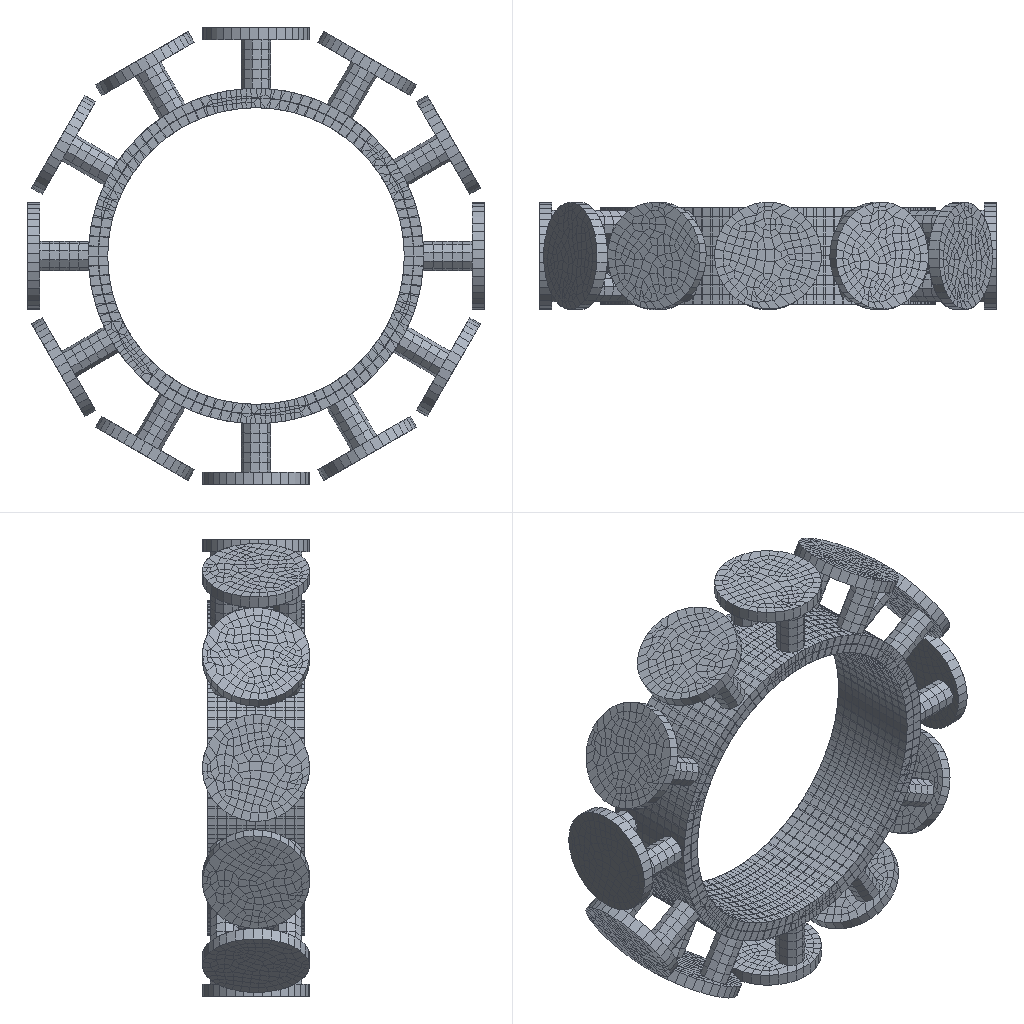Simulation study | abaqus
Set-up summary:
category,name,step,type,value,unit,region
solver,abaqus
solver,version,,,Abaqus/Explicit 2020
units,not stated in the deck,,not stated
analysis,deck,,transient,transient
load_step,Step-1,Step-1,transient
load_step,requested,,,1
mesh,nodes,,,21948
mesh,elements,,,16928
element_type,S4R,,shell,11811
element_type,C3D8R,,solid,5117
load,load commands in deck,,count,12
bc,support commands in deck,,count,5
material,CON,,in results
material,FRP,,in results
material,MATERIAL-3,,in results
check,setup vs results,,match,"per instance, exact: element labels, types and connectivity; labels of the nodes the elements use; coordinates of those nodes at SINGLE_PRECISION in 19 of 19 instance(s)"
Abaqus input file, long lists of numbers shortened:
*Heading
** Job name: Job-1 Model name: Model-1
** Generated by: Abaqus/CAE 2020
*Preprint, echo=NO, model=NO, history=NO, contact=NO
**
** PARTS
**
*Part, name=con
*Node
      1,         610.,   1219.589,           0.
      2,         650.,   1219.589,           0.
** (916 more lines like these left out)
*Element, type=C3D8R
  1,  10,  11,  14,  13,   1,   2,   5,   4
  2,  11,  12,  15,  14,   2,   3,   6,   5
** (406 more lines like these left out)
*Nset, nset=Set-1, generate
   1,  918,    1
*Elset, elset=Set-1, generate
   1,  408,    1
** Section: con
*Solid Section, elset=Set-1, material=con
,
*End Part
**
*Part, name=frp
*Node
      1,   666.024,    1000.002,           0.
      2,   666.024,    1160.002,           0.
** (8318 more lines like these left out)
*Element, type=S4R
   1,   48,   41,    6,    1
   2,   41,   42,    7,    6
** (8318 more lines like these left out)
*Nset, nset=Set-3, generate
    1,  8320,     1
*Elset, elset=Set-3, generate
    1,  8320,     1
** Section: Section-1
*Shell Section, elset=Set-3, material=frp
7., 5
*End Part
**
*Part, name=gangban
*Node
      1,         610.,   1059.589,           0.
      2,         610.,   979.589,           0.
** (3081 more lines like these left out)
*Element, type=S4R
  1,    1,   13, 1241,  108
  2,   13,   14, 1242, 1241
** (3489 more lines like these left out)
*Nset, nset=Set-3, generate
    1,  3083,     1
*Elset, elset=Set-3, generate
    1,  3491,     1
** Section: Section-1
*Shell Section, elset=Set-3, material=frp
7., 5
*End Part
**
*Part, name=m1
*Node
      1,         890.,   1007.07,  -46.852
      2,   688.407,   1007.07,  -46.852
** (478 more lines like these left out)
*Element, type=C3D8R
 1, 434, 437, 435, 433, 114, 117, 115, 113
 2, 438, 434, 433, 436, 118, 114, 113, 116
** (239 more lines like these left out)
*Nset, nset=Set-1, generate
   1,  480,    1
*Elset, elset=Set-1, generate
   1,  241,    1
** Section: m
*Solid Section, elset=Set-1, material=Material-3
,
*End Part
**
*Part, name=m2
*Node
      1,   747.337,   1007.07,  -485.575
      2,   572.752,   1007.07,   -384.779
** (516 more lines like these left out)
*Element, type=C3D8R
 1, 119,  12,  11, 120, 453, 130, 129, 454
 2, 114,  10,   9, 121, 448, 128, 127, 455
** (273 more lines like these left out)
*Nset, nset=Set-3, generate
   1,  518,    1
*Elset, elset=Set-3, generate
   1,  275,    1
** Section: m
*Solid Section, elset=Set-3, material=Material-3
,
*End Part
**
*Part, name=m3
*Node
      1,   404.425,   1007.07,   -794.189
      2,   303.629,   1007.07,  -619.604
** (537 more lines like these left out)
*Element, type=C3D8R
 1, 119,  12,  11, 120, 462, 130, 129, 463
 2, 114,  10,   9, 121, 457, 128, 127, 464
** (291 more lines like these left out)
*Nset, nset=Set-1, generate
   1,  539,    1
*Elset, elset=Set-1, generate
   1,  293,    1
** Section: m
*Solid Section, elset=Set-1, material=Material-3
,
*End Part
**
*Part, name=m4
*Node
      1,  -46.852,   1007.07,        -890.
      2,  -46.852,   1007.07,  -688.407
** (478 more lines like these left out)
*Element, type=C3D8R
 1, 434, 437, 435, 433, 114, 117, 115, 113
 2, 438, 434, 433, 436, 118, 114, 113, 116
** (239 more lines like these left out)
*Nset, nset=Set-1, generate
   1,  480,    1
*Elset, elset=Set-1, generate
   1,  241,    1
** Section: m
*Solid Section, elset=Set-1, material=Material-3
,
*End Part
**
*Part, name=m5
*Node
      1,  -485.575,   1007.07,  -747.337
      2,   -384.779,   1007.07,  -572.752
** (487 more lines like these left out)
*Element, type=C3D8R
 1, 430, 123, 124, 434, 113,   8,   9, 117
 2, 432, 437, 433, 431, 115, 120, 116, 114
** (251 more lines like these left out)
*Nset, nset=Set-1, generate
   1,  489,    1
*Elset, elset=Set-1, generate
   1,  253,    1
** Section: m
*Solid Section, elset=Set-1, material=Material-3
,
*End Part
**
*Part, name=m6
*Node
      1,   -794.189,   1007.07,  -404.425
      2,  -619.604,   1007.07,  -303.629
** (466 more lines like these left out)
*Element, type=C3D8R
 1, 429, 118, 119, 120, 113,   8,   9,  10
 2, 125, 431, 430, 124,  15, 115, 114,  14
** (228 more lines like these left out)
*Nset, nset=Set-1, generate
   1,  468,    1
*Elset, elset=Set-1, generate
   1,  230,    1
** Section: m
*Solid Section, elset=Set-1, material=Material-3
,
*End Part
**
*Part, name=m7
*Node
      1,        -890.,   1007.07,   46.852
      2,  -688.407,   1007.07,   46.852
** (462 more lines like these left out)
*Element, type=C3D8R
 1, 118, 119, 427, 425,   8,   9, 115, 113
 2, 428, 426, 425, 427, 116, 114, 113, 115
** (226 more lines like these left out)
*Nset, nset=Set-1, generate
   1,  464,    1
*Elset, elset=Set-1, generate
   1,  228,    1
** Section: m
*Solid Section, elset=Set-1, material=Material-3
,
*End Part
**
*Part, name=m8
*Node
      1,  -747.337,   1007.07,   485.575
      2,  -572.752,   1007.07,    384.779
** (516 more lines like these left out)
*Element, type=C3D8R
 1, 119,  12,  11, 120, 453, 130, 129, 454
 2,  10,   9, 121, 114, 128, 127, 455, 448
** (273 more lines like these left out)
*Nset, nset=Set-1, generate
   1,  518,    1
*Elset, elset=Set-1, generate
   1,  275,    1
** Section: m
*Solid Section, elset=Set-1, material=Material-3
,
*End Part
**
*Part, name=m9
*Node
      1,  -404.425,   1007.07,    794.189
      2,  -303.629,   1007.07,   619.604
** (468 more lines like these left out)
*Element, type=C3D8R
 1, 423, 120, 121, 426, 113,   8,   9, 116
 2, 428, 426, 123, 124, 118, 116,  11,  12
** (234 more lines like these left out)
*Nset, nset=Set-1, generate
   1,  470,    1
*Elset, elset=Set-1, generate
   1,  236,    1
** Section: m
*Solid Section, elset=Set-1, material=Material-3
,
*End Part
**
*Part, name=m10
*Node
      1,   46.852,   1007.07,         890.
      2,   46.852,   1007.07,   688.407
** (541 more lines like these left out)
*Element, type=C3D8R
 1, 113, 123, 119, 120, 460, 470, 466, 467
 2, 114,  10,   9, 121, 461, 128, 127, 468
** (293 more lines like these left out)
*Nset, nset=Set-1, generate
   1,  543,    1
*Elset, elset=Set-1, generate
   1,  295,    1
** Section: m
*Solid Section, elset=Set-1, material=Material-3
,
*End Part
**
*Part, name=m11
*Node
      1,   485.575,   1007.07,   747.337
      2,    384.779,   1007.07,   572.752
** (516 more lines like these left out)
*Element, type=C3D8R
 1, 119,  12,  11, 120, 453, 130, 129, 454
 2, 114,  10,   9, 121, 448, 128, 127, 455
** (273 more lines like these left out)
*Nset, nset=Set-1, generate
   1,  518,    1
*Elset, elset=Set-1, generate
   1,  275,    1
** Section: m
*Solid Section, elset=Set-1, material=Material-3
,
*End Part
**
*Part, name=m12
*Node
      1,    794.189,   1007.07,   404.425
      2,   619.604,   1007.07,   303.629
** (466 more lines like these left out)
*Element, type=C3D8R
 1, 421, 120, 121, 424, 113,   8,   9, 116
 2, 426, 424, 123, 124, 118, 116,  11,  12
** (233 more lines like these left out)
*Nset, nset=Set-1, generate
   1,  468,    1
*Elset, elset=Set-1, generate
   1,  235,    1
** Section: m
*Solid Section, elset=Set-1, material=Material-3
,
*End Part
**
**
** ASSEMBLY
**
*Assembly, name=Assembly
**
*Instance, name=con-1, part=con
*End Instance
**
*Instance, name=frp-1, part=frp
*End Instance
**
*Instance, name=gangban-1, part=gangban
*End Instance
**
*Instance, name=con-1-lin-1-2, part=con
          0.,         -80.,           0.
*End Instance
**
*Instance, name=con-1-lin-1-3, part=con
          0.,        -160.,           0.
*End Instance
**
*Instance, name=con-1-lin-1-4, part=con
          0.,        -240.,           0.
*End Instance
**
*Instance, name=con-1-lin-1-5, part=con
          0.,        -320.,           0.
*End Instance
**
*Instance, name=m1-1, part=m1
*End Instance
**
*Instance, name=m2-1, part=m2
*End Instance
**
*Instance, name=m3-1, part=m3
*End Instance
**
*Instance, name=m4-1, part=m4
*End Instance
**
*Instance, name=m5-1, part=m5
*End Instance
**
*Instance, name=m6-1, part=m6
*End Instance
**
*Instance, name=m7-1, part=m7
*End Instance
**
*Instance, name=m8-1, part=m8
*End Instance
**
*Instance, name=m9-1, part=m9
*End Instance
**
*Instance, name=m10-1, part=m10
*End Instance
**
*Instance, name=m11-1, part=m11
*End Instance
**
*Instance, name=m12-1, part=m12
*End Instance
**
*Node
      1,         470.,   1099.589,   814.064
*Node
      2,   814.064,   1099.589,         470.
*Node
      3,         940.,   1099.589, 1.34711146e-14
*Node
      4,   814.064,   1099.589,        -470.
*Node
      5,         470.,   1099.589,  -814.064
*Node
      6, 7.10295131e-14,   1099.589,        -940.
*Node
      7,        -470.,   1099.589,  -814.064
*Node
      8,  -814.064,   1099.589,        -470.
*Node
      9,        -940.,   1099.589, -1.28587909e-13
*Node
     10,  -814.064,   1099.589,         470.
*Node
     11,        -470.,   1099.589,   814.064
*Node
     12, -1.86146319e-13,   1099.589,         940.
*Node
     13,           0.,   1059.589, -3.73517271e-14
*Nset, nset=Set-3, instance=con-1
   7,   8,   9,  16,  17,  18,  25,  26,  27,  34,  35,  36,  43,  44,  45,  52
  53,  54,  61,  62,  63,  70,  71,  72,  79,  80,  81,  88,  89,  90,  97,  98
** (18 more lines like these left out)
*Elset, elset=Set-3, instance=con-1
   3,   4,   7,   8,  11,  12,  15,  16,  19,  20,  23,  24,  27,  28,  31,  32
  35,  36,  39,  40,  43,  44,  47,  48,  51,  52,  55,  56,  59,  60,  63,  64
** (11 more lines like these left out)
*Nset, nset=Set-4, instance=m1-1
   4,   5,  34,  35,  36,  37,  38,  39,  40,  41,  42,  43,  44,  45,  46,  47
  48,  49,  50,  51,  52,  53,  54,  55,  56,  57,  58,  59,  60,  61,  62,  63
** (3 more lines like these left out)
*Nset, nset=Set-4, instance=m2-1
   4,   5,  34,  35,  36,  37,  38,  39,  40,  41,  42,  43,  44,  45,  46,  47
  48,  49,  50,  51,  52,  53,  54,  55,  56,  57,  58,  59,  60,  61,  62,  63
** (3 more lines like these left out)
*Nset, nset=Set-4, instance=m4-1
   4,   5,  34,  35,  36,  37,  38,  39,  40,  41,  42,  43,  44,  45,  46,  47
  48,  49,  50,  51,  52,  53,  54,  55,  56,  57,  58,  59,  60,  61,  62,  63
** (3 more lines like these left out)
*Nset, nset=Set-4, instance=m6-1
   4,   5,  34,  35,  36,  37,  38,  39,  40,  41,  42,  43,  44,  45,  46,  47
  48,  49,  50,  51,  52,  53,  54,  55,  56,  57,  58,  59,  60,  61,  62,  63
** (3 more lines like these left out)
*Nset, nset=Set-4, instance=m10-1
   4,   5,  34,  35,  36,  37,  38,  39,  40,  41,  42,  43,  44,  45,  46,  47
  48,  49,  50,  51,  52,  53,  54,  55,  56,  57,  58,  59,  60,  61,  62,  63
** (3 more lines like these left out)
*Nset, nset=Set-4, instance=m8-1
   4,   5,  34,  35,  36,  37,  38,  39,  40,  41,  42,  43,  44,  45,  46,  47
  48,  49,  50,  51,  52,  53,  54,  55,  56,  57,  58,  59,  60,  61,  62,  63
** (3 more lines like these left out)
*Nset, nset=Set-4, instance=m12-1
   4,   5,  34,  35,  36,  37,  38,  39,  40,  41,  42,  43,  44,  45,  46,  47
  48,  49,  50,  51,  52,  53,  54,  55,  56,  57,  58,  59,  60,  61,  62,  63
** (3 more lines like these left out)
*Nset, nset=Set-4, instance=m3-1
   4,   5,  34,  35,  36,  37,  38,  39,  40,  41,  42,  43,  44,  45,  46,  47
  48,  49,  50,  51,  52,  53,  54,  55,  56,  57,  58,  59,  60,  61,  62,  63
** (3 more lines like these left out)
*Nset, nset=Set-4, instance=m7-1
   4,   5,  34,  35,  36,  37,  38,  39,  40,  41,  42,  43,  44,  45,  46,  47
  48,  49,  50,  51,  52,  53,  54,  55,  56,  57,  58,  59,  60,  61,  62,  63
** (3 more lines like these left out)
*Nset, nset=Set-4, instance=m11-1
   4,   5,  34,  35,  36,  37,  38,  39,  40,  41,  42,  43,  44,  45,  46,  47
  48,  49,  50,  51,  52,  53,  54,  55,  56,  57,  58,  59,  60,  61,  62,  63
** (3 more lines like these left out)
*Nset, nset=Set-4, instance=m5-1
   4,   5,  34,  35,  36,  37,  38,  39,  40,  41,  42,  43,  44,  45,  46,  47
  48,  49,  50,  51,  52,  53,  54,  55,  56,  57,  58,  59,  60,  61,  62,  63
** (3 more lines like these left out)
*Nset, nset=Set-4, instance=m9-1
   4,   5,  34,  35,  36,  37,  38,  39,  40,  41,  42,  43,  44,  45,  46,  47
  48,  49,  50,  51,  52,  53,  54,  55,  56,  57,  58,  59,  60,  61,  62,  63
** (3 more lines like these left out)
*Elset, elset=Set-4, instance=m1-1
  77,  80,  82,  83,  84,  86,  88,  90,  91,  92,  98,  99, 100, 104, 105, 106
 107, 109, 111, 112, 113, 116, 118, 122, 129, 130, 131, 132, 133, 134, 136, 137
** (1 more lines like these left out)
*Elset, elset=Set-4, instance=m2-1
 101, 106, 107, 108, 109, 110, 111, 112, 113, 115, 117, 122, 123, 130, 131, 132
 133, 134, 138, 141, 143, 147, 153, 154, 156, 157, 158, 159, 160, 161, 164, 165
** (1 more lines like these left out)
*Elset, elset=Set-4, instance=m4-1
  77,  80,  82,  83,  84,  87,  89,  91,  92,  93,  99, 100, 101, 104, 105, 106
 107, 109, 111, 112, 113, 116, 117, 121, 129, 130, 131, 132, 133, 134, 136, 137
** (1 more lines like these left out)
*Elset, elset=Set-4, instance=m6-1
  52,  53,  61,  62,  66,  67,  68,  70,  71,  72,  73,  74,  76,  80,  84,  88
  89,  92,  93,  94,  97, 101, 107, 112, 113, 114, 117, 118, 119, 121, 122, 124
** (1 more lines like these left out)
*Elset, elset=Set-4, instance=m10-1
 103, 111, 112, 114, 115, 116, 118, 120, 123, 124, 126, 131, 133, 137, 138, 139
 140, 142, 145, 148, 150, 153, 160, 161, 162, 163, 164, 165, 166, 167, 168, 170
** (1 more lines like these left out)
*Elset, elset=Set-4, instance=m8-1
 100, 105, 106, 107, 108, 109, 110, 111, 112, 113, 115, 120, 121, 122, 130, 131
 133, 134, 138, 142, 145, 153, 154, 155, 156, 157, 158, 159, 161, 162, 165, 166
** (1 more lines like these left out)
*Elset, elset=Set-4, instance=m12-1
  62,  63,  71,  75,  76,  77,  79,  80,  81,  82,  83,  85,  89,  91,  94,  97
  98, 101, 102, 103, 106, 110, 115, 122, 123, 124, 125, 126, 129, 130, 134, 135
** (1 more lines like these left out)
*Elset, elset=Set-4, instance=m3-1
  95,  96, 104, 109, 110, 111, 113, 114, 115, 116, 118, 123, 124, 127, 131, 132
 135, 136, 138, 141, 145, 149, 153, 158, 159, 161, 162, 163, 165, 166, 168, 169
** (1 more lines like these left out)
*Elset, elset=Set-4, instance=m7-1
  67,  70,  72,  73,  74,  77,  79,  81,  82,  83,  89,  90,  91,  94,  95,  96
  97,  99, 100, 101, 102, 105, 106, 111, 118, 119, 120, 122, 123, 124, 126, 127
** (1 more lines like these left out)
*Elset, elset=Set-4, instance=m11-1
 101, 106, 107, 109, 110, 111, 112, 113, 115, 117, 122, 123, 124, 131, 132, 133
 134, 138, 141, 145, 147, 152, 153, 154, 155, 157, 159, 160, 161, 162, 165, 166
** (1 more lines like these left out)
*Elset, elset=Set-4, instance=m5-1
  86,  91,  92,  93,  94,  96,  97,  98, 100, 102, 106, 115, 116, 117, 118, 119
 121, 124, 126, 133, 137, 138, 140, 141, 142, 143, 144, 145, 146, 147, 151, 152
** (1 more lines like these left out)
*Elset, elset=Set-4, instance=m9-1
  62,  63,  71,  75,  76,  77,  78,  80,  81,  82,  83,  85,  87,  91,  93,  99
 100, 103, 104, 105, 108, 112, 117, 120, 124, 125, 126, 127, 130, 131, 135, 136
** (1 more lines like these left out)
*Nset, nset=Set-30
 13,
*Nset, nset=b_Set-5, instance=m11-1, generate
   1,  518,    1
*Elset, elset=b_Set-5, instance=m11-1, generate
   1,  275,    1
*Nset, nset=b_Set-7, instance=m12-1, generate
   1,  468,    1
*Elset, elset=b_Set-7, instance=m12-1, generate
   1,  235,    1
*Nset, nset=b_Set-9, instance=m1-1, generate
   1,  480,    1
*Elset, elset=b_Set-9, instance=m1-1, generate
   1,  241,    1
*Nset, nset=b_Set-11, instance=m2-1, generate
   1,  518,    1
*Elset, elset=b_Set-11, instance=m2-1, generate
   1,  275,    1
*Nset, nset=b_Set-13, instance=m3-1, generate
   1,  539,    1
*Elset, elset=b_Set-13, instance=m3-1, generate
   1,  293,    1
*Nset, nset=b_Set-15, instance=m4-1, generate
   1,  480,    1
*Elset, elset=b_Set-15, instance=m4-1, generate
   1,  241,    1
*Nset, nset=b_Set-17, instance=m5-1, generate
   1,  489,    1
*Elset, elset=b_Set-17, instance=m5-1, generate
   1,  253,    1
*Nset, nset=b_Set-19, instance=m6-1, generate
   1,  468,    1
*Elset, elset=b_Set-19, instance=m6-1, generate
   1,  230,    1
*Nset, nset=b_Set-21, instance=m7-1, generate
   1,  464,    1
*Elset, elset=b_Set-21, instance=m7-1, generate
   1,  228,    1
*Nset, nset=b_Set-23, instance=m8-1, generate
   1,  518,    1
*Elset, elset=b_Set-23, instance=m8-1, generate
   1,  275,    1
*Nset, nset=b_Set-25, instance=m9-1, generate
   1,  470,    1
*Elset, elset=b_Set-25, instance=m9-1, generate
   1,  236,    1
*Nset, nset=b_Set-27, instance=m10-1, generate
   1,  543,    1
*Elset, elset=b_Set-27, instance=m10-1, generate
   1,  295,    1
*Nset, nset=m_Set-1, instance=frp-1, generate
    1,  8320,     1
*Elset, elset=m_Set-1, instance=frp-1, generate
    1,  8320,     1
*Nset, nset=m_Set-29
 13,
*Nset, nset=s_Set-1, instance=con-1, generate
   1,  918,    1
*Nset, nset=s_Set-1, instance=con-1-lin-1-2, generate
   1,  918,    1
*Nset, nset=s_Set-1, instance=con-1-lin-1-3, generate
   1,  918,    1
*Nset, nset=s_Set-1, instance=con-1-lin-1-5, generate
   1,  918,    1
*Nset, nset=s_Set-1, instance=con-1-lin-1-4, generate
   1,  918,    1
*Elset, elset=s_Set-1, instance=con-1, generate
   1,  408,    1
*Elset, elset=s_Set-1, instance=con-1-lin-1-2, generate
   1,  408,    1
*Elset, elset=s_Set-1, instance=con-1-lin-1-3, generate
   1,  408,    1
*Elset, elset=s_Set-1, instance=con-1-lin-1-5, generate
   1,  408,    1
*Elset, elset=s_Set-1, instance=con-1-lin-1-4, generate
   1,  408,    1
*Nset, nset=_PickedSet98, internal
 1,
*Nset, nset=_PickedSet100, internal
 2,
*Nset, nset=_PickedSet102, internal
 3,
*Nset, nset=_PickedSet104, internal
 4,
*Nset, nset=_PickedSet106, internal
 5,
*Nset, nset=_PickedSet108, internal
 6,
*Nset, nset=_PickedSet110, internal
 7,
*Nset, nset=_PickedSet112, internal
 8,
*Nset, nset=_PickedSet114, internal
 9,
*Nset, nset=_PickedSet116, internal
 10,
*Nset, nset=_PickedSet118, internal
 11,
*Nset, nset=_PickedSet120, internal
 12,
*Elset, elset=_Surf-1_S1, internal, instance=m10-1, generate
  81,  214,    1
*Elset, elset=_Surf-1_S2, internal, instance=m10-1, generate
 215,  230,    1
*Surface, type=ELEMENT, name=Surf-1
_Surf-1_S1, S1
_Surf-1_S2, S2
*Elset, elset=_Surf-2_S2, internal, instance=m9-1
  51,  52,  53,  54,  55,  56,  57,  58,  59,  60, 177, 178, 179, 180, 181, 182
 183, 184, 185, 186
*Elset, elset=_Surf-2_S1, internal, instance=m9-1, generate
  61,  176,    1
*Surface, type=ELEMENT, name=Surf-2
_Surf-2_S2, S2
_Surf-2_S1, S1
*Elset, elset=_Surf-3_S1, internal, instance=m8-1, generate
  81,  209,    1
*Elset, elset=_Surf-3_S2, internal, instance=m8-1, generate
 210,  225,    1
*Surface, type=ELEMENT, name=Surf-3
_Surf-3_S1, S1
_Surf-3_S2, S2
*Elset, elset=_Surf-4_S2, internal, instance=m7-1
  41,  42,  43,  44,  45,  46,  47,  48,  49,  50, 171, 172, 173, 174, 175, 176
 177, 178
*Elset, elset=_Surf-4_S1, internal, instance=m7-1, generate
  51,  170,    1
*Surface, type=ELEMENT, name=Surf-4
_Surf-4_S2, S2
_Surf-4_S1, S1
*Elset, elset=_Surf-5_S2, internal, instance=m6-1
  41,  42,  43,  44,  45,  46,  47,  48,  49,  50, 173, 174, 175, 176, 177, 178
 179, 180
*Elset, elset=_Surf-5_S1, internal, instance=m6-1, generate
  51,  172,    1
*Surface, type=ELEMENT, name=Surf-5
_Surf-5_S2, S2
_Surf-5_S1, S1
*Elset, elset=_Surf-6_S2, internal, instance=m5-1
  66,  67,  68,  69,  70,  71,  72,  73,  74,  75, 191, 192, 193, 194, 195, 196
 197, 198, 199, 200, 201, 202, 203
*Elset, elset=_Surf-6_S1, internal, instance=m5-1, generate
  76,  190,    1
*Surface, type=ELEMENT, name=Surf-6
_Surf-6_S2, S2
_Surf-6_S1, S1
*Elset, elset=_Surf-7_S2, internal, instance=m4-1
  51,  52,  53,  54,  55,  56,  57,  58,  59,  60, 182, 183, 184, 185, 186, 187
 188, 189, 190, 191
*Elset, elset=_Surf-7_S1, internal, instance=m4-1, generate
  61,  181,    1
*Surface, type=ELEMENT, name=Surf-7
_Surf-7_S2, S2
_Surf-7_S1, S1
*Elset, elset=_Surf-8_S1, internal, instance=m3-1, generate
  81,  212,    1
*Elset, elset=_Surf-8_S2, internal, instance=m3-1, generate
 213,  228,    1
*Surface, type=ELEMENT, name=Surf-8
_Surf-8_S1, S1
_Surf-8_S2, S2
*Elset, elset=_Surf-9_S1, internal, instance=m2-1, generate
  81,  209,    1
*Elset, elset=_Surf-9_S2, internal, instance=m2-1, generate
 210,  225,    1
*Surface, type=ELEMENT, name=Surf-9
_Surf-9_S1, S1
_Surf-9_S2, S2
*Elset, elset=_Surf-10_S2, internal, instance=m1-1
  51,  52,  53,  54,  55,  56,  57,  58,  59,  60, 182, 183, 184, 185, 186, 187
 188, 189, 190, 191
*Elset, elset=_Surf-10_S1, internal, instance=m1-1, generate
  61,  181,    1
*Surface, type=ELEMENT, name=Surf-10
_Surf-10_S2, S2
_Surf-10_S1, S1
*Elset, elset=_Surf-11_S2, internal, instance=m12-1
  51,  52,  53,  54,  55,  56,  57,  58,  59,  60, 176, 177, 178, 179, 180, 181
 182, 183, 184, 185
*Elset, elset=_Surf-11_S1, internal, instance=m12-1, generate
  61,  175,    1
*Surface, type=ELEMENT, name=Surf-11
_Surf-11_S2, S2
_Surf-11_S1, S1
*Elset, elset=_Surf-12_S1, internal, instance=m11-1, generate
  81,  209,    1
*Elset, elset=_Surf-12_S2, internal, instance=m11-1, generate
 210,  225,    1
*Surface, type=ELEMENT, name=Surf-12
_Surf-12_S1, S1
_Surf-12_S2, S2
*Elset, elset=_s_Surf-14_SPOS, internal, instance=gangban-1, generate
 3017,  3491,     1
*Surface, type=ELEMENT, name=s_Surf-14
_s_Surf-14_SPOS, SPOS
*Elset, elset=_shuchu_SPOS, internal, instance=gangban-1
  193,  194,  195,  196,  197,  198,  199,  200,  201,  202,  203,  204,  205,  206,  207,  208
  209,  210,  211,  212,  213,  214,  215,  216,  217,  218,  219,  220,  221,  222,  223,  224
** (66 more lines like these left out)
*Surface, type=ELEMENT, name=shuchu
_shuchu_SPOS, SPOS
** Constraint: Constraint-1
*Embedded Element, host elset=s_Set-1
m_Set-1
** Constraint: Constraint-2
*Rigid Body, ref node=_PickedSet98, elset=b_Set-5
** Constraint: Constraint-3
*Rigid Body, ref node=_PickedSet100, elset=b_Set-7
** Constraint: Constraint-4
*Rigid Body, ref node=_PickedSet102, elset=b_Set-9
** Constraint: Constraint-5
*Rigid Body, ref node=_PickedSet104, elset=b_Set-11
** Constraint: Constraint-6
*Rigid Body, ref node=_PickedSet106, elset=b_Set-13
** Constraint: Constraint-7
*Rigid Body, ref node=_PickedSet108, elset=b_Set-15
** Constraint: Constraint-8
*Rigid Body, ref node=_PickedSet110, elset=b_Set-17
** Constraint: Constraint-9
*Rigid Body, ref node=_PickedSet112, elset=b_Set-19
** Constraint: Constraint-10
*Rigid Body, ref node=_PickedSet114, elset=b_Set-21
** Constraint: Constraint-11
*Rigid Body, ref node=_PickedSet116, elset=b_Set-23
** Constraint: Constraint-12
*Rigid Body, ref node=_PickedSet118, elset=b_Set-25
** Constraint: Constraint-13
*Rigid Body, ref node=_PickedSet120, elset=b_Set-27
** Constraint: Constraint-SHUCHU
*Coupling, constraint name=Constraint-SHUCHU, ref node=m_Set-29, surface=s_Surf-14
*Kinematic
*End Assembly
*Amplitude, name=Amp-1
             0.,              0.,             0.5,              1.
**
** MATERIALS
**
*Material, name=Material-3
*Density
 7.8e-09,
*Elastic
180000., 0.3
*Plastic
347.,0.
*Material, name=con
*Density
 2.2e-09,
*Elastic
35900., 0.22
*Plastic
60.,0.
*Material, name=frp
*Density
 1.5e-09,
*Elastic, type=ENGINEERING CONSTANTS
11810.,11200.,11810.,  0.24,  0.23,  0.23, 7800., 8900.
 8900.,
**
** INTERACTION PROPERTIES
**
*Surface Interaction, name=IntProp-1
*Friction
 0.2,
*Surface Behavior, pressure-overclosure=HARD
**
** INTERACTIONS
**
** Interaction: Int-1
*Contact, op=NEW
*Contact Inclusions, ALL EXTERIOR
*Contact Property Assignment
 ,  , IntProp-1
** ----------------------------------------------------------------
**
** STEP: Step-1
**
*Step, name=Step-1, nlgeom=YES
*Dynamic, Explicit
, 0.5
*Bulk Viscosity
0.06, 1.2
** Mass Scaling: Semi-Automatic
**               Whole Model
*Fixed Mass Scaling, factor=50.
**
** BOUNDARY CONDITIONS
**
** Name: BC-2 Type: 位移/转角
*Boundary
Set-4, 2, 2
Set-4, 4, 4
Set-4, 5, 5
Set-4, 6, 6
** Name: BC-3 Type: 对称/反对称/完全固定
*Boundary
Set-30, ENCASTRE
**
** LOADS
**
** Name: Load-1   Type: Pressure
*Dsload
Surf-1, P, 0.01058
** Name: Load-2   Type: Pressure
*Dsload
Surf-2, P, 0.01084
** Name: Load-3   Type: Pressure
*Dsload
Surf-3, P, 0.01217
** Name: Load-4   Type: Pressure
*Dsload
Surf-4, P, 0.01126
** Name: Load-5   Type: Pressure
*Dsload
Surf-5, P, 0.0113
** Name: Load-6   Type: Pressure
*Dsload
Surf-6, P, 0.0107
** Name: Load-7   Type: Pressure
*Dsload
Surf-7, P, 0.012
** Name: Load-8   Type: Pressure
*Dsload
Surf-8, P, 0.01236
** Name: Load-9   Type: Pressure
*Dsload
Surf-9, P, 0.01305
** Name: Load-10   Type: Pressure
*Dsload
Surf-10, P, 0.0124
** Name: Load-11   Type: Pressure
*Dsload
Surf-11, P, 0.01184
** Name: Load-12   Type: Pressure
*Dsload
Surf-12, P, 0.01114
**
** OUTPUT REQUESTS
**
*Restart, write, number interval=1, time marks=NO
**
** FIELD OUTPUT: F-Output-1
**
*Output, field, number interval=50
*Node Output
A, CF, RF, RM, RT, U, V
*Element Output, directions=YES
E, LE, MISES, MISESMAX, MISESONLY, PE, PEEQ, PEEQVAVG, PEVAVG, S, SF, SSAVG, SVAVG
*Contact Output
CDISP, CSTRESS
**
** HISTORY OUTPUT: H-Output-1
**
*Output, history, time interval=5e-06
*Node Output, nset=Set-30
RF1, RF3, U1, U3
*End Step
Results summary:
result,step,Step-1,completed,increments=13070 time=0.5/0.5
result,analysis,,,transient
result,last_loadstep,,,1
result,primary field,,,"U, UR"
result,reaction total,,FX,326.554,model units
result,reaction total,,FY,-279.11,model units
result,reaction total,,FZ,-268.814,model units